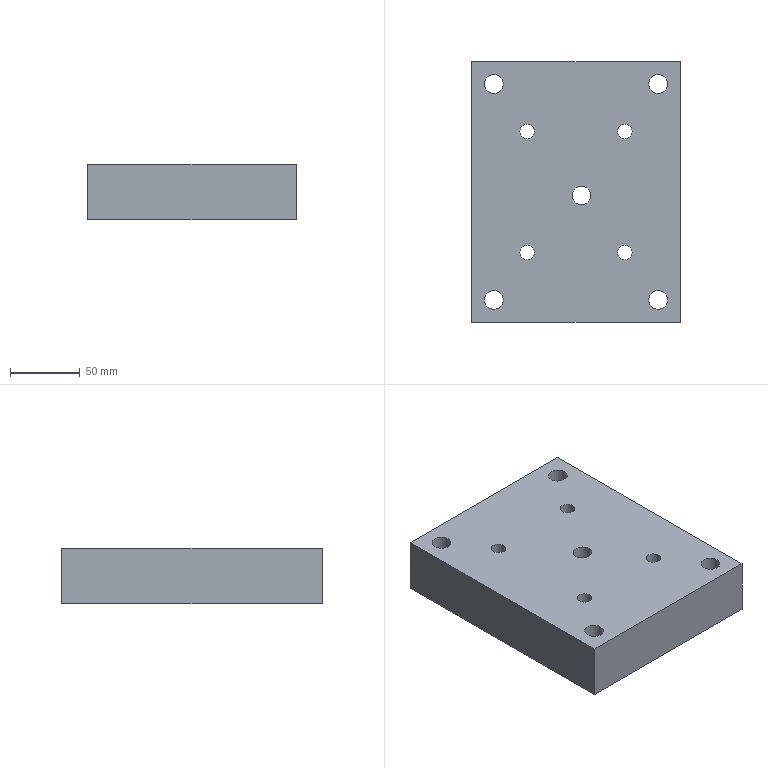Part | STEP file | lll_id2198_x_t | 1 solid | 47 faces | box 150 x 187 x 40 mm | volume 927967 mm3 | cylinder 24 | plane 21 | cone 2 | commonest cylinder face diameters 10 x8 13.509 x5 20.007 x5 10.506 x4 10.505 x2
STEP:
#1=CARTESIAN_POINT('',(2920.,63.439,117.5));
#2=VERTEX_POINT('',#1);
#3=CARTESIAN_POINT('',(2928.371,68.5,117.5));
#4=VERTEX_POINT('',#3);
#5=CARTESIAN_POINT('',(2923.648,66.859,117.5));
#6=DIRECTION('',(0.,0.,-1.));
#7=DIRECTION('',(-1.,0.,0.));
#8=AXIS2_PLACEMENT_3D('',#5,#6,#7);
#9=CIRCLE('',#8,5.);
#10=EDGE_CURVE('',#2,#4,#9,.T.);
#11=ORIENTED_EDGE('',*,*,#10,.F.);
#12=CARTESIAN_POINT('',(2920.,28.561,117.5));
#13=VERTEX_POINT('',#12);
#14=CARTESIAN_POINT('',(2920.,0.00007422,117.5));
#15=DIRECTION('',(0.,1.,0.));
#16=VECTOR('',#15,1.);
#17=LINE('',#14,#16);
#18=EDGE_CURVE('',#13,#2,#17,.T.);
#19=ORIENTED_EDGE('',*,*,#18,.F.);
#20=CARTESIAN_POINT('',(2928.371,23.5,117.5));
#21=VERTEX_POINT('',#20);
#22=CARTESIAN_POINT('',(2923.648,25.142,117.5));
#23=DIRECTION('',(0.,0.,-1.));
#24=DIRECTION('',(-1.,0.,0.));
#25=AXIS2_PLACEMENT_3D('',#22,#23,#24);
#26=CIRCLE('',#25,5.);
#27=EDGE_CURVE('',#21,#13,#26,.T.);
#28=ORIENTED_EDGE('',*,*,#27,.F.);
#29=CARTESIAN_POINT('',(3011.629,23.5,117.5));
#30=VERTEX_POINT('',#29);
#31=CARTESIAN_POINT('',(2970.,23.5,117.5));
#32=DIRECTION('',(-1.,0.,0.));
#33=VECTOR('',#32,1.);
#34=LINE('',#31,#33);
#35=EDGE_CURVE('',#30,#21,#34,.T.);
#36=ORIENTED_EDGE('',*,*,#35,.F.);
#37=CARTESIAN_POINT('',(3020.,28.561,117.5));
#38=VERTEX_POINT('',#37);
#39=CARTESIAN_POINT('',(3016.352,25.142,117.5));
#40=DIRECTION('',(0.,0.,-1.));
#41=DIRECTION('',(-1.,0.,0.));
#42=AXIS2_PLACEMENT_3D('',#39,#40,#41);
#43=CIRCLE('',#42,5.);
#44=EDGE_CURVE('',#38,#30,#43,.T.);
#45=ORIENTED_EDGE('',*,*,#44,.F.);
#46=CARTESIAN_POINT('',(3020.,63.439,117.5));
#47=VERTEX_POINT('',#46);
#48=CARTESIAN_POINT('',(3020.,0.00007422,117.5));
#49=DIRECTION('',(0.,-1.,0.));
#50=VECTOR('',#49,1.);
#51=LINE('',#48,#50);
#52=EDGE_CURVE('',#47,#38,#51,.T.);
#53=ORIENTED_EDGE('',*,*,#52,.F.);
#54=CARTESIAN_POINT('',(3011.629,68.5,117.5));
#55=VERTEX_POINT('',#54);
#56=CARTESIAN_POINT('',(3016.352,66.859,117.5));
#57=DIRECTION('',(0.,0.,-1.));
#58=DIRECTION('',(-1.,0.,0.));
#59=AXIS2_PLACEMENT_3D('',#56,#57,#58);
#60=CIRCLE('',#59,5.);
#61=EDGE_CURVE('',#55,#47,#60,.T.);
#62=ORIENTED_EDGE('',*,*,#61,.F.);
#63=CARTESIAN_POINT('',(2970.,68.5,117.5));
#64=DIRECTION('',(1.,0.,0.));
#65=VECTOR('',#64,1.);
#66=LINE('',#63,#65);
#67=EDGE_CURVE('',#4,#55,#66,.T.);
#68=ORIENTED_EDGE('',*,*,#67,.F.);
#69=EDGE_LOOP('',(#11,#19,#28,#36,#45,#53,#62,#68));
#70=FACE_BOUND('',#69,.T.);
#71=CARTESIAN_POINT('',(2920.,-28.561,117.5));
#72=VERTEX_POINT('',#71);
#73=CARTESIAN_POINT('',(2928.371,-23.5,117.5));
#74=VERTEX_POINT('',#73);
#75=CARTESIAN_POINT('',(2923.648,-25.141,117.5));
#76=DIRECTION('',(0.,0.,-1.));
#77=DIRECTION('',(-1.,0.,0.));
#78=AXIS2_PLACEMENT_3D('',#75,#76,#77);
#79=CIRCLE('',#78,5.);
#80=EDGE_CURVE('',#72,#74,#79,.T.);
#81=ORIENTED_EDGE('',*,*,#80,.F.);
#82=CARTESIAN_POINT('',(2920.,-63.439,117.5));
#83=VERTEX_POINT('',#82);
#84=CARTESIAN_POINT('',(2920.,0.00007422,117.5));
#85=DIRECTION('',(0.,1.,0.));
#86=VECTOR('',#85,1.);
#87=LINE('',#84,#86);
#88=EDGE_CURVE('',#83,#72,#87,.T.);
#89=ORIENTED_EDGE('',*,*,#88,.F.);
#90=CARTESIAN_POINT('',(2928.371,-68.5,117.5));
#91=VERTEX_POINT('',#90);
#92=CARTESIAN_POINT('',(2923.648,-66.858,117.5));
#93=DIRECTION('',(0.,0.,-1.));
#94=DIRECTION('',(-1.,0.,0.));
#95=AXIS2_PLACEMENT_3D('',#92,#93,#94);
#96=CIRCLE('',#95,5.);
#97=EDGE_CURVE('',#91,#83,#96,.T.);
#98=ORIENTED_EDGE('',*,*,#97,.F.);
#99=CARTESIAN_POINT('',(3011.629,-68.5,117.5));
#100=VERTEX_POINT('',#99);
#101=CARTESIAN_POINT('',(2970.,-68.5,117.5));
#102=DIRECTION('',(-1.,0.,0.));
#103=VECTOR('',#102,1.);
#104=LINE('',#101,#103);
#105=EDGE_CURVE('',#100,#91,#104,.T.);
#106=ORIENTED_EDGE('',*,*,#105,.F.);
#107=CARTESIAN_POINT('',(3020.,-63.439,117.5));
#108=VERTEX_POINT('',#107);
#109=CARTESIAN_POINT('',(3016.352,-66.858,117.5));
#110=DIRECTION('',(0.,0.,-1.));
#111=DIRECTION('',(-1.,0.,0.));
#112=AXIS2_PLACEMENT_3D('',#109,#110,#111);
#113=CIRCLE('',#112,5.);
#114=EDGE_CURVE('',#108,#100,#113,.T.);
#115=ORIENTED_EDGE('',*,*,#114,.F.);
#116=CARTESIAN_POINT('',(3020.,-28.561,117.5));
#117=VERTEX_POINT('',#116);
#118=CARTESIAN_POINT('',(3020.,0.00007422,117.5));
#119=DIRECTION('',(0.,-1.,0.));
#120=VECTOR('',#119,1.);
#121=LINE('',#118,#120);
#122=EDGE_CURVE('',#117,#108,#121,.T.);
#123=ORIENTED_EDGE('',*,*,#122,.F.);
#124=CARTESIAN_POINT('',(3011.629,-23.5,117.5));
#125=VERTEX_POINT('',#124);
#126=CARTESIAN_POINT('',(3016.352,-25.141,117.5));
#127=DIRECTION('',(0.,0.,-1.));
#128=DIRECTION('',(-1.,0.,0.));
#129=AXIS2_PLACEMENT_3D('',#126,#127,#128);
#130=CIRCLE('',#129,5.);
#131=EDGE_CURVE('',#125,#117,#130,.T.);
#132=ORIENTED_EDGE('',*,*,#131,.F.);
#133=CARTESIAN_POINT('',(2970.,-23.5,117.5));
#134=DIRECTION('',(1.,0.,0.));
#135=VECTOR('',#134,1.);
#136=LINE('',#133,#135);
#137=EDGE_CURVE('',#74,#125,#136,.T.);
#138=ORIENTED_EDGE('',*,*,#137,.F.);
#139=EDGE_LOOP('',(#81,#89,#98,#106,#115,#123,#132,#138));
#140=FACE_BOUND('',#139,.T.);
#141=CARTESIAN_POINT('',(2935.747,77.5,117.5));
#142=VERTEX_POINT('',#141);
#143=CARTESIAN_POINT('',(2941.,77.5,117.5));
#144=DIRECTION('',(0.,0.,-1.));
#145=DIRECTION('',(-1.,0.,0.));
#146=AXIS2_PLACEMENT_3D('',#143,#144,#145);
#147=CIRCLE('',#146,5.253);
#148=EDGE_CURVE('',#142,#142,#147,.T.);
#149=ORIENTED_EDGE('',*,*,#148,.F.);
#150=EDGE_LOOP('',(#149));
#151=FACE_BOUND('',#150,.T.);
#152=CARTESIAN_POINT('',(3039.003,77.5,117.5));
#153=VERTEX_POINT('',#152);
#154=CARTESIAN_POINT('',(3029.,77.5,117.5));
#155=DIRECTION('',(0.,0.,1.));
#156=DIRECTION('',(1.,0.,0.));
#157=AXIS2_PLACEMENT_3D('',#154,#155,#156);
#158=CIRCLE('',#157,10.004);
#159=EDGE_CURVE('',#153,#153,#158,.T.);
#160=ORIENTED_EDGE('',*,*,#159,.T.);
#161=EDGE_LOOP('',(#160));
#162=FACE_BOUND('',#161,.T.);
#163=CARTESIAN_POINT('',(2921.003,-77.5,117.5));
#164=VERTEX_POINT('',#163);
#165=CARTESIAN_POINT('',(2911.,-77.5,117.5));
#166=DIRECTION('',(0.,0.,1.));
#167=DIRECTION('',(1.,0.,0.));
#168=AXIS2_PLACEMENT_3D('',#165,#166,#167);
#169=CIRCLE('',#168,10.004);
#170=EDGE_CURVE('',#164,#164,#169,.T.);
#171=ORIENTED_EDGE('',*,*,#170,.T.);
#172=EDGE_LOOP('',(#171));
#173=FACE_BOUND('',#172,.T.);
#174=CARTESIAN_POINT('',(2993.747,-77.5,117.5));
#175=VERTEX_POINT('',#174);
#176=CARTESIAN_POINT('',(2999.,-77.5,117.5));
#177=DIRECTION('',(0.,0.,-1.));
#178=DIRECTION('',(-1.,0.,0.));
#179=AXIS2_PLACEMENT_3D('',#176,#177,#178);
#180=CIRCLE('',#179,5.253);
#181=EDGE_CURVE('',#175,#175,#180,.T.);
#182=ORIENTED_EDGE('',*,*,#181,.F.);
#183=EDGE_LOOP('',(#182));
#184=FACE_BOUND('',#183,.T.);
#185=CARTESIAN_POINT('',(3045.,-93.5,117.5));
#186=VERTEX_POINT('',#185);
#187=CARTESIAN_POINT('',(3045.,93.5,117.5));
#188=VERTEX_POINT('',#187);
#189=CARTESIAN_POINT('',(3045.,0.00007422,117.5));
#190=DIRECTION('',(0.,1.,0.));
#191=VECTOR('',#190,1.);
#192=LINE('',#189,#191);
#193=EDGE_CURVE('',#186,#188,#192,.T.);
#194=ORIENTED_EDGE('',*,*,#193,.F.);
#195=CARTESIAN_POINT('',(2895.,-93.5,117.5));
#196=VERTEX_POINT('',#195);
#197=CARTESIAN_POINT('',(2970.,-93.5,117.5));
#198=DIRECTION('',(1.,0.,0.));
#199=VECTOR('',#198,1.);
#200=LINE('',#197,#199);
#201=EDGE_CURVE('',#196,#186,#200,.T.);
#202=ORIENTED_EDGE('',*,*,#201,.F.);
#203=CARTESIAN_POINT('',(2895.,93.5,117.5));
#204=VERTEX_POINT('',#203);
#205=CARTESIAN_POINT('',(2895.,0.00007422,117.5));
#206=DIRECTION('',(0.,-1.,0.));
#207=VECTOR('',#206,1.);
#208=LINE('',#205,#207);
#209=EDGE_CURVE('',#204,#196,#208,.T.);
#210=ORIENTED_EDGE('',*,*,#209,.F.);
#211=CARTESIAN_POINT('',(2970.,93.5,117.5));
#212=DIRECTION('',(-1.,0.,0.));
#213=VECTOR('',#212,1.);
#214=LINE('',#211,#213);
#215=EDGE_CURVE('',#188,#204,#214,.T.);
#216=ORIENTED_EDGE('',*,*,#215,.F.);
#217=EDGE_LOOP('',(#194,#202,#210,#216));
#218=FACE_BOUND('',#217,.T.);
#219=CARTESIAN_POINT('',(3039.003,-77.5,117.5));
#220=VERTEX_POINT('',#219);
#221=CARTESIAN_POINT('',(3029.,-77.5,117.5));
#222=DIRECTION('',(0.,0.,1.));
#223=DIRECTION('',(1.,0.,0.));
#224=AXIS2_PLACEMENT_3D('',#221,#222,#223);
#225=CIRCLE('',#224,10.004);
#226=EDGE_CURVE('',#220,#220,#225,.T.);
#227=ORIENTED_EDGE('',*,*,#226,.T.);
#228=EDGE_LOOP('',(#227));
#229=FACE_BOUND('',#228,.T.);
#230=CARTESIAN_POINT('',(2984.003,-2.5,117.5));
#231=VERTEX_POINT('',#230);
#232=CARTESIAN_POINT('',(2974.,-2.5,117.5));
#233=DIRECTION('',(0.,0.,1.));
#234=DIRECTION('',(1.,0.,0.));
#235=AXIS2_PLACEMENT_3D('',#232,#233,#234);
#236=CIRCLE('',#235,10.004);
#237=EDGE_CURVE('',#231,#231,#236,.T.);
#238=ORIENTED_EDGE('',*,*,#237,.T.);
#239=EDGE_LOOP('',(#238));
#240=FACE_BOUND('',#239,.T.);
#241=CARTESIAN_POINT('',(2921.003,77.5,117.5));
#242=VERTEX_POINT('',#241);
#243=CARTESIAN_POINT('',(2911.,77.5,117.5));
#244=DIRECTION('',(0.,0.,1.));
#245=DIRECTION('',(1.,0.,0.));
#246=AXIS2_PLACEMENT_3D('',#243,#244,#245);
#247=CIRCLE('',#246,10.004);
#248=EDGE_CURVE('',#242,#242,#247,.T.);
#249=ORIENTED_EDGE('',*,*,#248,.T.);
#250=EDGE_LOOP('',(#249));
#251=FACE_BOUND('',#250,.T.);
#252=CARTESIAN_POINT('',(2970.,0.00007422,117.5));
#253=DIRECTION('',(0.,0.,-1.));
#254=DIRECTION('',(-1.,0.,0.));
#255=AXIS2_PLACEMENT_3D('',#252,#253,#254);
#256=PLANE('',#255);
#257=ADVANCED_FACE('',(#70,#140,#151,#162,#173,#184,#218,#229,#240,#251),#256,.T.);
#258=CARTESIAN_POINT('',(2999.747,43.5,157.5));
#259=VERTEX_POINT('',#258);
#260=CARTESIAN_POINT('',(3005.,43.5,157.5));
#261=DIRECTION('',(0.,0.,-1.));
#262=DIRECTION('',(-1.,0.,0.));
#263=AXIS2_PLACEMENT_3D('',#260,#261,#262);
#264=CIRCLE('',#263,5.253);
#265=EDGE_CURVE('',#259,#259,#264,.T.);
#266=ORIENTED_EDGE('',*,*,#265,.T.);
#267=EDGE_LOOP('',(#266));
#268=FACE_BOUND('',#267,.T.);
#269=CARTESIAN_POINT('',(2929.747,43.5,157.5));
#270=VERTEX_POINT('',#269);
#271=CARTESIAN_POINT('',(2935.,43.5,157.5));
#272=DIRECTION('',(0.,0.,-1.));
#273=DIRECTION('',(-1.,0.,0.));
#274=AXIS2_PLACEMENT_3D('',#271,#272,#273);
#275=CIRCLE('',#274,5.253);
#276=EDGE_CURVE('',#270,#270,#275,.T.);
#277=ORIENTED_EDGE('',*,*,#276,.T.);
#278=EDGE_LOOP('',(#277));
#279=FACE_BOUND('',#278,.T.);
#280=CARTESIAN_POINT('',(2999.747,-43.5,157.5));
#281=VERTEX_POINT('',#280);
#282=CARTESIAN_POINT('',(3005.,-43.5,157.5));
#283=DIRECTION('',(0.,0.,-1.));
#284=DIRECTION('',(-1.,0.,0.));
#285=AXIS2_PLACEMENT_3D('',#282,#283,#284);
#286=CIRCLE('',#285,5.253);
#287=EDGE_CURVE('',#281,#281,#286,.T.);
#288=ORIENTED_EDGE('',*,*,#287,.T.);
#289=EDGE_LOOP('',(#288));
#290=FACE_BOUND('',#289,.T.);
#291=CARTESIAN_POINT('',(2929.747,-43.5,157.5));
#292=VERTEX_POINT('',#291);
#293=CARTESIAN_POINT('',(2935.,-43.5,157.5));
#294=DIRECTION('',(0.,0.,-1.));
#295=DIRECTION('',(-1.,0.,0.));
#296=AXIS2_PLACEMENT_3D('',#293,#294,#295);
#297=CIRCLE('',#296,5.253);
#298=EDGE_CURVE('',#292,#292,#297,.T.);
#299=ORIENTED_EDGE('',*,*,#298,.T.);
#300=EDGE_LOOP('',(#299));
#301=FACE_BOUND('',#300,.T.);
#302=CARTESIAN_POINT('',(2904.245,77.5,157.5));
#303=VERTEX_POINT('',#302);
#304=CARTESIAN_POINT('',(2911.,77.5,157.5));
#305=DIRECTION('',(0.,0.,1.));
#306=DIRECTION('',(-1.,0.,0.));
#307=AXIS2_PLACEMENT_3D('',#304,#305,#306);
#308=CIRCLE('',#307,6.755);
#309=EDGE_CURVE('',#303,#303,#308,.T.);
#310=ORIENTED_EDGE('',*,*,#309,.F.);
#311=EDGE_LOOP('',(#310));
#312=FACE_BOUND('',#311,.T.);
#313=CARTESIAN_POINT('',(3022.245,77.5,157.5));
#314=VERTEX_POINT('',#313);
#315=CARTESIAN_POINT('',(3029.,77.5,157.5));
#316=DIRECTION('',(0.,0.,1.));
#317=DIRECTION('',(-1.,0.,0.));
#318=AXIS2_PLACEMENT_3D('',#315,#316,#317);
#319=CIRCLE('',#318,6.755);
#320=EDGE_CURVE('',#314,#314,#319,.T.);
#321=ORIENTED_EDGE('',*,*,#320,.F.);
#322=EDGE_LOOP('',(#321));
#323=FACE_BOUND('',#322,.T.);
#324=CARTESIAN_POINT('',(2967.245,-2.5,157.5));
#325=VERTEX_POINT('',#324);
#326=CARTESIAN_POINT('',(2974.,-2.5,157.5));
#327=DIRECTION('',(0.,0.,1.));
#328=DIRECTION('',(-1.,0.,0.));
#329=AXIS2_PLACEMENT_3D('',#326,#327,#328);
#330=CIRCLE('',#329,6.755);
#331=EDGE_CURVE('',#325,#325,#330,.T.);
#332=ORIENTED_EDGE('',*,*,#331,.F.);
#333=EDGE_LOOP('',(#332));
#334=FACE_BOUND('',#333,.T.);
#335=CARTESIAN_POINT('',(2904.245,-77.5,157.5));
#336=VERTEX_POINT('',#335);
#337=CARTESIAN_POINT('',(2911.,-77.5,157.5));
#338=DIRECTION('',(0.,0.,1.));
#339=DIRECTION('',(-1.,0.,0.));
#340=AXIS2_PLACEMENT_3D('',#337,#338,#339);
#341=CIRCLE('',#340,6.755);
#342=EDGE_CURVE('',#336,#336,#341,.T.);
#343=ORIENTED_EDGE('',*,*,#342,.F.);
#344=EDGE_LOOP('',(#343));
#345=FACE_BOUND('',#344,.T.);
#346=CARTESIAN_POINT('',(3022.245,-77.5,157.5));
#347=VERTEX_POINT('',#346);
#348=CARTESIAN_POINT('',(3029.,-77.5,157.5));
#349=DIRECTION('',(0.,0.,1.));
#350=DIRECTION('',(-1.,0.,0.));
#351=AXIS2_PLACEMENT_3D('',#348,#349,#350);
#352=CIRCLE('',#351,6.755);
#353=EDGE_CURVE('',#347,#347,#352,.T.);
#354=ORIENTED_EDGE('',*,*,#353,.F.);
#355=EDGE_LOOP('',(#354));
#356=FACE_BOUND('',#355,.T.);
#357=CARTESIAN_POINT('',(3045.,-93.5,157.5));
#358=VERTEX_POINT('',#357);
#359=CARTESIAN_POINT('',(2895.,-93.5,157.5));
#360=VERTEX_POINT('',#359);
#361=CARTESIAN_POINT('',(2970.,-93.5,157.5));
#362=DIRECTION('',(-1.,0.,0.));
#363=VECTOR('',#362,1.);
#364=LINE('',#361,#363);
#365=EDGE_CURVE('',#358,#360,#364,.T.);
#366=ORIENTED_EDGE('',*,*,#365,.F.);
#367=CARTESIAN_POINT('',(3045.,93.5,157.5));
#368=VERTEX_POINT('',#367);
#369=CARTESIAN_POINT('',(3045.,0.00007422,157.5));
#370=DIRECTION('',(0.,-1.,0.));
#371=VECTOR('',#370,1.);
#372=LINE('',#369,#371);
#373=EDGE_CURVE('',#368,#358,#372,.T.);
#374=ORIENTED_EDGE('',*,*,#373,.F.);
#375=CARTESIAN_POINT('',(2895.,93.5,157.5));
#376=VERTEX_POINT('',#375);
#377=CARTESIAN_POINT('',(2970.,93.5,157.5));
#378=DIRECTION('',(1.,0.,0.));
#379=VECTOR('',#378,1.);
#380=LINE('',#377,#379);
#381=EDGE_CURVE('',#376,#368,#380,.T.);
#382=ORIENTED_EDGE('',*,*,#381,.F.);
#383=CARTESIAN_POINT('',(2895.,0.00007422,157.5));
#384=DIRECTION('',(0.,1.,0.));
#385=VECTOR('',#384,1.);
#386=LINE('',#383,#385);
#387=EDGE_CURVE('',#360,#376,#386,.T.);
#388=ORIENTED_EDGE('',*,*,#387,.F.);
#389=EDGE_LOOP('',(#366,#374,#382,#388));
#390=FACE_BOUND('',#389,.T.);
#391=CARTESIAN_POINT('',(-2196.249,0.,157.5));
#392=DIRECTION('',(0.,0.,-1.));
#393=DIRECTION('',(1.,0.,0.));
#394=AXIS2_PLACEMENT_3D('',#391,#392,#393);
#395=PLANE('',#394);
#396=ADVANCED_FACE('',(#268,#279,#290,#301,#312,#323,#334,#345,#356,#390),#395,.F.);
#397=CARTESIAN_POINT('',(3045.,-93.5,127.5));
#398=DIRECTION('',(0.,0.,1.));
#399=VECTOR('',#398,1.);
#400=LINE('',#397,#399);
#401=EDGE_CURVE('',#186,#358,#400,.T.);
#402=ORIENTED_EDGE('',*,*,#401,.T.);
#403=ORIENTED_EDGE('',*,*,#365,.T.);
#404=CARTESIAN_POINT('',(2895.,-93.5,127.5));
#405=DIRECTION('',(0.,0.,1.));
#406=VECTOR('',#405,1.);
#407=LINE('',#404,#406);
#408=EDGE_CURVE('',#196,#360,#407,.T.);
#409=ORIENTED_EDGE('',*,*,#408,.F.);
#410=ORIENTED_EDGE('',*,*,#201,.T.);
#411=EDGE_LOOP('',(#402,#403,#409,#410));
#412=FACE_OUTER_BOUND('',#411,.T.);
#413=CARTESIAN_POINT('',(2970.,-93.5,127.5));
#414=DIRECTION('',(0.,-1.,0.));
#415=DIRECTION('',(0.,0.,-1.));
#416=AXIS2_PLACEMENT_3D('',#413,#414,#415);
#417=PLANE('',#416);
#418=ADVANCED_FACE('',(#412),#417,.T.);
#419=ORIENTED_EDGE('',*,*,#408,.T.);
#420=ORIENTED_EDGE('',*,*,#387,.T.);
#421=CARTESIAN_POINT('',(2895.,93.5,127.5));
#422=DIRECTION('',(0.,0.,1.));
#423=VECTOR('',#422,1.);
#424=LINE('',#421,#423);
#425=EDGE_CURVE('',#204,#376,#424,.T.);
#426=ORIENTED_EDGE('',*,*,#425,.F.);
#427=ORIENTED_EDGE('',*,*,#209,.T.);
#428=EDGE_LOOP('',(#419,#420,#426,#427));
#429=FACE_OUTER_BOUND('',#428,.T.);
#430=CARTESIAN_POINT('',(2895.,0.00007422,127.5));
#431=DIRECTION('',(-1.,0.,0.));
#432=DIRECTION('',(0.,0.,1.));
#433=AXIS2_PLACEMENT_3D('',#430,#431,#432);
#434=PLANE('',#433);
#435=ADVANCED_FACE('',(#429),#434,.T.);
#436=ORIENTED_EDGE('',*,*,#425,.T.);
#437=ORIENTED_EDGE('',*,*,#381,.T.);
#438=CARTESIAN_POINT('',(3045.,93.5,127.5));
#439=DIRECTION('',(0.,0.,1.));
#440=VECTOR('',#439,1.);
#441=LINE('',#438,#440);
#442=EDGE_CURVE('',#188,#368,#441,.T.);
#443=ORIENTED_EDGE('',*,*,#442,.F.);
#444=ORIENTED_EDGE('',*,*,#215,.T.);
#445=EDGE_LOOP('',(#436,#437,#443,#444));
#446=FACE_OUTER_BOUND('',#445,.T.);
#447=CARTESIAN_POINT('',(2970.,93.5,127.5));
#448=DIRECTION('',(0.,1.,0.));
#449=DIRECTION('',(0.,0.,1.));
#450=AXIS2_PLACEMENT_3D('',#447,#448,#449);
#451=PLANE('',#450);
#452=ADVANCED_FACE('',(#446),#451,.T.);
#453=ORIENTED_EDGE('',*,*,#193,.T.);
#454=ORIENTED_EDGE('',*,*,#442,.T.);
#455=ORIENTED_EDGE('',*,*,#373,.T.);
#456=ORIENTED_EDGE('',*,*,#401,.F.);
#457=EDGE_LOOP('',(#453,#454,#455,#456));
#458=FACE_OUTER_BOUND('',#457,.T.);
#459=CARTESIAN_POINT('',(3045.,0.00007422,127.5));
#460=DIRECTION('',(1.,0.,0.));
#461=DIRECTION('',(0.,0.,-1.));
#462=AXIS2_PLACEMENT_3D('',#459,#460,#461);
#463=PLANE('',#462);
#464=ADVANCED_FACE('',(#458),#463,.T.);
#465=ORIENTED_EDGE('',*,*,#353,.T.);
#466=EDGE_LOOP('',(#465));
#467=FACE_BOUND('',#466,.T.);
#468=CARTESIAN_POINT('',(3035.755,-77.5,132.5));
#469=VERTEX_POINT('',#468);
#470=CARTESIAN_POINT('',(3029.,-77.5,132.5));
#471=DIRECTION('',(0.,0.,1.));
#472=DIRECTION('',(1.,0.,0.));
#473=AXIS2_PLACEMENT_3D('',#470,#471,#472);
#474=CIRCLE('',#473,6.755);
#475=EDGE_CURVE('',#469,#469,#474,.T.);
#476=ORIENTED_EDGE('',*,*,#475,.F.);
#477=EDGE_LOOP('',(#476));
#478=FACE_BOUND('',#477,.T.);
#479=CARTESIAN_POINT('',(3029.,-77.5,112.5));
#480=DIRECTION('',(0.,0.,1.));
#481=DIRECTION('',(1.,0.,0.));
#482=AXIS2_PLACEMENT_3D('',#479,#480,#481);
#483=CYLINDRICAL_SURFACE('',#482,6.755);
#484=ADVANCED_FACE('',(#467,#478),#483,.F.);
#485=ORIENTED_EDGE('',*,*,#475,.T.);
#486=EDGE_LOOP('',(#485));
#487=FACE_BOUND('',#486,.T.);
#488=CARTESIAN_POINT('',(3039.003,-77.5,132.5));
#489=VERTEX_POINT('',#488);
#490=CARTESIAN_POINT('',(3029.,-77.5,132.5));
#491=DIRECTION('',(0.,0.,1.));
#492=DIRECTION('',(1.,0.,0.));
#493=AXIS2_PLACEMENT_3D('',#490,#491,#492);
#494=CIRCLE('',#493,10.004);
#495=EDGE_CURVE('',#489,#489,#494,.T.);
#496=ORIENTED_EDGE('',*,*,#495,.F.);
#497=EDGE_LOOP('',(#496));
#498=FACE_BOUND('',#497,.T.);
#499=CARTESIAN_POINT('',(3029.,-77.5,132.5));
#500=DIRECTION('',(0.,0.,1.));
#501=DIRECTION('',(1.,0.,0.));
#502=AXIS2_PLACEMENT_3D('',#499,#500,#501);
#503=PLANE('',#502);
#504=ADVANCED_FACE('',(#487,#498),#503,.F.);
#505=ORIENTED_EDGE('',*,*,#495,.T.);
#506=EDGE_LOOP('',(#505));
#507=FACE_BOUND('',#506,.T.);
#508=ORIENTED_EDGE('',*,*,#226,.F.);
#509=EDGE_LOOP('',(#508));
#510=FACE_BOUND('',#509,.T.);
#511=CARTESIAN_POINT('',(3029.,-77.5,117.5));
#512=DIRECTION('',(0.,0.,1.));
#513=DIRECTION('',(1.,0.,0.));
#514=AXIS2_PLACEMENT_3D('',#511,#512,#513);
#515=CYLINDRICAL_SURFACE('',#514,10.004);
#516=ADVANCED_FACE('',(#507,#510),#515,.F.);
#517=ORIENTED_EDGE('',*,*,#181,.T.);
#518=EDGE_LOOP('',(#517));
#519=FACE_BOUND('',#518,.T.);
#520=CARTESIAN_POINT('',(3004.253,-77.5,147.254));
#521=VERTEX_POINT('',#520);
#522=CARTESIAN_POINT('',(2999.,-77.5,147.254));
#523=DIRECTION('',(0.,0.,1.));
#524=DIRECTION('',(1.,0.,0.));
#525=AXIS2_PLACEMENT_3D('',#522,#523,#524);
#526=CIRCLE('',#525,5.253);
#527=EDGE_CURVE('',#521,#521,#526,.T.);
#528=ORIENTED_EDGE('',*,*,#527,.T.);
#529=EDGE_LOOP('',(#528));
#530=FACE_BOUND('',#529,.T.);
#531=CARTESIAN_POINT('',(2999.,-77.5,112.5));
#532=DIRECTION('',(0.,0.,1.));
#533=DIRECTION('',(1.,0.,0.));
#534=AXIS2_PLACEMENT_3D('',#531,#532,#533);
#535=CYLINDRICAL_SURFACE('',#534,5.253);
#536=ADVANCED_FACE('',(#519,#530),#535,.F.);
#537=CARTESIAN_POINT('',(2999.,-77.5,152.506));
#538=VERTEX_POINT('',#537);
#539=VERTEX_LOOP('',#538);
#540=FACE_BOUND('',#539,.T.);
#541=ORIENTED_EDGE('',*,*,#527,.F.);
#542=EDGE_LOOP('',(#541));
#543=FACE_BOUND('',#542,.T.);
#544=CARTESIAN_POINT('',(2999.,-77.5,147.254));
#545=DIRECTION('',(0.,0.,-1.));
#546=DIRECTION('',(-1.,0.,0.));
#547=AXIS2_PLACEMENT_3D('',#544,#545,#546);
#548=CONICAL_SURFACE('',#547,5.253,45.);
#549=ADVANCED_FACE('',(#540,#543),#548,.F.);
#550=ORIENTED_EDGE('',*,*,#342,.T.);
#551=EDGE_LOOP('',(#550));
#552=FACE_BOUND('',#551,.T.);
#553=CARTESIAN_POINT('',(2917.755,-77.5,132.5));
#554=VERTEX_POINT('',#553);
#555=CARTESIAN_POINT('',(2911.,-77.5,132.5));
#556=DIRECTION('',(0.,0.,1.));
#557=DIRECTION('',(1.,0.,0.));
#558=AXIS2_PLACEMENT_3D('',#555,#556,#557);
#559=CIRCLE('',#558,6.755);
#560=EDGE_CURVE('',#554,#554,#559,.T.);
#561=ORIENTED_EDGE('',*,*,#560,.F.);
#562=EDGE_LOOP('',(#561));
#563=FACE_BOUND('',#562,.T.);
#564=CARTESIAN_POINT('',(2911.,-77.5,112.5));
#565=DIRECTION('',(0.,0.,1.));
#566=DIRECTION('',(1.,0.,0.));
#567=AXIS2_PLACEMENT_3D('',#564,#565,#566);
#568=CYLINDRICAL_SURFACE('',#567,6.755);
#569=ADVANCED_FACE('',(#552,#563),#568,.F.);
#570=ORIENTED_EDGE('',*,*,#560,.T.);
#571=EDGE_LOOP('',(#570));
#572=FACE_BOUND('',#571,.T.);
#573=CARTESIAN_POINT('',(2921.003,-77.5,132.5));
#574=VERTEX_POINT('',#573);
#575=CARTESIAN_POINT('',(2911.,-77.5,132.5));
#576=DIRECTION('',(0.,0.,1.));
#577=DIRECTION('',(1.,0.,0.));
#578=AXIS2_PLACEMENT_3D('',#575,#576,#577);
#579=CIRCLE('',#578,10.004);
#580=EDGE_CURVE('',#574,#574,#579,.T.);
#581=ORIENTED_EDGE('',*,*,#580,.F.);
#582=EDGE_LOOP('',(#581));
#583=FACE_BOUND('',#582,.T.);
#584=CARTESIAN_POINT('',(2911.,-77.5,132.5));
#585=DIRECTION('',(0.,0.,1.));
#586=DIRECTION('',(1.,0.,0.));
#587=AXIS2_PLACEMENT_3D('',#584,#585,#586);
#588=PLANE('',#587);
#589=ADVANCED_FACE('',(#572,#583),#588,.F.);
#590=ORIENTED_EDGE('',*,*,#580,.T.);
#591=EDGE_LOOP('',(#590));
#592=FACE_BOUND('',#591,.T.);
#593=ORIENTED_EDGE('',*,*,#170,.F.);
#594=EDGE_LOOP('',(#593));
#595=FACE_BOUND('',#594,.T.);
#596=CARTESIAN_POINT('',(2911.,-77.5,117.5));
#597=DIRECTION('',(0.,0.,1.));
#598=DIRECTION('',(1.,0.,0.));
#599=AXIS2_PLACEMENT_3D('',#596,#597,#598);
#600=CYLINDRICAL_SURFACE('',#599,10.004);
#601=ADVANCED_FACE('',(#592,#595),#600,.F.);
#602=ORIENTED_EDGE('',*,*,#331,.T.);
#603=EDGE_LOOP('',(#602));
#604=FACE_BOUND('',#603,.T.);
#605=CARTESIAN_POINT('',(2980.755,-2.5,132.5));
#606=VERTEX_POINT('',#605);
#607=CARTESIAN_POINT('',(2974.,-2.5,132.5));
#608=DIRECTION('',(0.,0.,1.));
#609=DIRECTION('',(1.,0.,0.));
#610=AXIS2_PLACEMENT_3D('',#607,#608,#609);
#611=CIRCLE('',#610,6.755);
#612=EDGE_CURVE('',#606,#606,#611,.T.);
#613=ORIENTED_EDGE('',*,*,#612,.F.);
#614=EDGE_LOOP('',(#613));
#615=FACE_BOUND('',#614,.T.);
#616=CARTESIAN_POINT('',(2974.,-2.5,112.5));
#617=DIRECTION('',(0.,0.,1.));
#618=DIRECTION('',(1.,0.,0.));
#619=AXIS2_PLACEMENT_3D('',#616,#617,#618);
#620=CYLINDRICAL_SURFACE('',#619,6.755);
#621=ADVANCED_FACE('',(#604,#615),#620,.F.);
#622=ORIENTED_EDGE('',*,*,#612,.T.);
#623=EDGE_LOOP('',(#622));
#624=FACE_BOUND('',#623,.T.);
#625=CARTESIAN_POINT('',(2984.003,-2.5,132.5));
#626=VERTEX_POINT('',#625);
#627=CARTESIAN_POINT('',(2974.,-2.5,132.5));
#628=DIRECTION('',(0.,0.,1.));
#629=DIRECTION('',(1.,0.,0.));
#630=AXIS2_PLACEMENT_3D('',#627,#628,#629);
#631=CIRCLE('',#630,10.004);
#632=EDGE_CURVE('',#626,#626,#631,.T.);
#633=ORIENTED_EDGE('',*,*,#632,.F.);
#634=EDGE_LOOP('',(#633));
#635=FACE_BOUND('',#634,.T.);
#636=CARTESIAN_POINT('',(2974.,-2.5,132.5));
#637=DIRECTION('',(0.,0.,1.));
#638=DIRECTION('',(1.,0.,0.));
#639=AXIS2_PLACEMENT_3D('',#636,#637,#638);
#640=PLANE('',#639);
#641=ADVANCED_FACE('',(#624,#635),#640,.F.);
#642=ORIENTED_EDGE('',*,*,#632,.T.);
#643=EDGE_LOOP('',(#642));
#644=FACE_BOUND('',#643,.T.);
#645=ORIENTED_EDGE('',*,*,#237,.F.);
#646=EDGE_LOOP('',(#645));
#647=FACE_BOUND('',#646,.T.);
#648=CARTESIAN_POINT('',(2974.,-2.5,117.5));
#649=DIRECTION('',(0.,0.,1.));
#650=DIRECTION('',(1.,0.,0.));
#651=AXIS2_PLACEMENT_3D('',#648,#649,#650);
#652=CYLINDRICAL_SURFACE('',#651,10.004);
#653=ADVANCED_FACE('',(#644,#647),#652,.F.);
#654=ORIENTED_EDGE('',*,*,#320,.T.);
#655=EDGE_LOOP('',(#654));
#656=FACE_BOUND('',#655,.T.);
#657=CARTESIAN_POINT('',(3035.755,77.5,132.5));
#658=VERTEX_POINT('',#657);
#659=CARTESIAN_POINT('',(3029.,77.5,132.5));
#660=DIRECTION('',(0.,0.,1.));
#661=DIRECTION('',(1.,0.,0.));
#662=AXIS2_PLACEMENT_3D('',#659,#660,#661);
#663=CIRCLE('',#662,6.755);
#664=EDGE_CURVE('',#658,#658,#663,.T.);
#665=ORIENTED_EDGE('',*,*,#664,.F.);
#666=EDGE_LOOP('',(#665));
#667=FACE_BOUND('',#666,.T.);
#668=CARTESIAN_POINT('',(3029.,77.5,112.5));
#669=DIRECTION('',(0.,0.,1.));
#670=DIRECTION('',(1.,0.,0.));
#671=AXIS2_PLACEMENT_3D('',#668,#669,#670);
#672=CYLINDRICAL_SURFACE('',#671,6.755);
#673=ADVANCED_FACE('',(#656,#667),#672,.F.);
#674=ORIENTED_EDGE('',*,*,#664,.T.);
#675=EDGE_LOOP('',(#674));
#676=FACE_BOUND('',#675,.T.);
#677=CARTESIAN_POINT('',(3039.003,77.5,132.5));
#678=VERTEX_POINT('',#677);
#679=CARTESIAN_POINT('',(3029.,77.5,132.5));
#680=DIRECTION('',(0.,0.,1.));
#681=DIRECTION('',(1.,0.,0.));
#682=AXIS2_PLACEMENT_3D('',#679,#680,#681);
#683=CIRCLE('',#682,10.004);
#684=EDGE_CURVE('',#678,#678,#683,.T.);
#685=ORIENTED_EDGE('',*,*,#684,.F.);
#686=EDGE_LOOP('',(#685));
#687=FACE_BOUND('',#686,.T.);
#688=CARTESIAN_POINT('',(3029.,77.5,132.5));
#689=DIRECTION('',(0.,0.,1.));
#690=DIRECTION('',(1.,0.,0.));
#691=AXIS2_PLACEMENT_3D('',#688,#689,#690);
#692=PLANE('',#691);
#693=ADVANCED_FACE('',(#676,#687),#692,.F.);
#694=ORIENTED_EDGE('',*,*,#684,.T.);
#695=EDGE_LOOP('',(#694));
#696=FACE_BOUND('',#695,.T.);
#697=ORIENTED_EDGE('',*,*,#159,.F.);
#698=EDGE_LOOP('',(#697));
#699=FACE_BOUND('',#698,.T.);
#700=CARTESIAN_POINT('',(3029.,77.5,117.5));
#701=DIRECTION('',(0.,0.,1.));
#702=DIRECTION('',(1.,0.,0.));
#703=AXIS2_PLACEMENT_3D('',#700,#701,#702);
#704=CYLINDRICAL_SURFACE('',#703,10.004);
#705=ADVANCED_FACE('',(#696,#699),#704,.F.);
#706=ORIENTED_EDGE('',*,*,#309,.T.);
#707=EDGE_LOOP('',(#706));
#708=FACE_BOUND('',#707,.T.);
#709=CARTESIAN_POINT('',(2917.755,77.5,132.5));
#710=VERTEX_POINT('',#709);
#711=CARTESIAN_POINT('',(2911.,77.5,132.5));
#712=DIRECTION('',(0.,0.,1.));
#713=DIRECTION('',(1.,0.,0.));
#714=AXIS2_PLACEMENT_3D('',#711,#712,#713);
#715=CIRCLE('',#714,6.755);
#716=EDGE_CURVE('',#710,#710,#715,.T.);
#717=ORIENTED_EDGE('',*,*,#716,.F.);
#718=EDGE_LOOP('',(#717));
#719=FACE_BOUND('',#718,.T.);
#720=CARTESIAN_POINT('',(2911.,77.5,112.5));
#721=DIRECTION('',(0.,0.,1.));
#722=DIRECTION('',(1.,0.,0.));
#723=AXIS2_PLACEMENT_3D('',#720,#721,#722);
#724=CYLINDRICAL_SURFACE('',#723,6.755);
#725=ADVANCED_FACE('',(#708,#719),#724,.F.);
#726=ORIENTED_EDGE('',*,*,#716,.T.);
#727=EDGE_LOOP('',(#726));
#728=FACE_BOUND('',#727,.T.);
#729=CARTESIAN_POINT('',(2921.003,77.5,132.5));
#730=VERTEX_POINT('',#729);
#731=CARTESIAN_POINT('',(2911.,77.5,132.5));
#732=DIRECTION('',(0.,0.,1.));
#733=DIRECTION('',(1.,0.,0.));
#734=AXIS2_PLACEMENT_3D('',#731,#732,#733);
#735=CIRCLE('',#734,10.004);
#736=EDGE_CURVE('',#730,#730,#735,.T.);
#737=ORIENTED_EDGE('',*,*,#736,.F.);
#738=EDGE_LOOP('',(#737));
#739=FACE_BOUND('',#738,.T.);
#740=CARTESIAN_POINT('',(2911.,77.5,132.5));
#741=DIRECTION('',(0.,0.,1.));
#742=DIRECTION('',(1.,0.,0.));
#743=AXIS2_PLACEMENT_3D('',#740,#741,#742);
#744=PLANE('',#743);
#745=ADVANCED_FACE('',(#728,#739),#744,.F.);
#746=ORIENTED_EDGE('',*,*,#736,.T.);
#747=EDGE_LOOP('',(#746));
#748=FACE_BOUND('',#747,.T.);
#749=ORIENTED_EDGE('',*,*,#248,.F.);
#750=EDGE_LOOP('',(#749));
#751=FACE_BOUND('',#750,.T.);
#752=CARTESIAN_POINT('',(2911.,77.5,117.5));
#753=DIRECTION('',(0.,0.,1.));
#754=DIRECTION('',(1.,0.,0.));
#755=AXIS2_PLACEMENT_3D('',#752,#753,#754);
#756=CYLINDRICAL_SURFACE('',#755,10.004);
#757=ADVANCED_FACE('',(#748,#751),#756,.F.);
#758=ORIENTED_EDGE('',*,*,#148,.T.);
#759=EDGE_LOOP('',(#758));
#760=FACE_BOUND('',#759,.T.);
#761=CARTESIAN_POINT('',(2946.253,77.5,147.254));
#762=VERTEX_POINT('',#761);
#763=CARTESIAN_POINT('',(2941.,77.5,147.254));
#764=DIRECTION('',(0.,0.,1.));
#765=DIRECTION('',(1.,0.,0.));
#766=AXIS2_PLACEMENT_3D('',#763,#764,#765);
#767=CIRCLE('',#766,5.253);
#768=EDGE_CURVE('',#762,#762,#767,.T.);
#769=ORIENTED_EDGE('',*,*,#768,.T.);
#770=EDGE_LOOP('',(#769));
#771=FACE_BOUND('',#770,.T.);
#772=CARTESIAN_POINT('',(2941.,77.5,112.5));
#773=DIRECTION('',(0.,0.,1.));
#774=DIRECTION('',(1.,0.,0.));
#775=AXIS2_PLACEMENT_3D('',#772,#773,#774);
#776=CYLINDRICAL_SURFACE('',#775,5.253);
#777=ADVANCED_FACE('',(#760,#771),#776,.F.);
#778=CARTESIAN_POINT('',(2941.,77.5,152.506));
#779=VERTEX_POINT('',#778);
#780=VERTEX_LOOP('',#779);
#781=FACE_BOUND('',#780,.T.);
#782=ORIENTED_EDGE('',*,*,#768,.F.);
#783=EDGE_LOOP('',(#782));
#784=FACE_BOUND('',#783,.T.);
#785=CARTESIAN_POINT('',(2941.,77.5,147.254));
#786=DIRECTION('',(0.,0.,-1.));
#787=DIRECTION('',(-1.,0.,0.));
#788=AXIS2_PLACEMENT_3D('',#785,#786,#787);
#789=CONICAL_SURFACE('',#788,5.253,45.);
#790=ADVANCED_FACE('',(#781,#784),#789,.F.);
#791=CARTESIAN_POINT('',(3010.253,-43.5,132.5));
#792=VERTEX_POINT('',#791);
#793=CARTESIAN_POINT('',(3005.,-43.5,132.5));
#794=DIRECTION('',(0.,0.,1.));
#795=DIRECTION('',(1.,0.,0.));
#796=AXIS2_PLACEMENT_3D('',#793,#794,#795);
#797=CIRCLE('',#796,5.253);
#798=EDGE_CURVE('',#792,#792,#797,.T.);
#799=ORIENTED_EDGE('',*,*,#798,.T.);
#800=EDGE_LOOP('',(#799));
#801=FACE_BOUND('',#800,.T.);
#802=CARTESIAN_POINT('',(2940.253,-43.5,132.5));
#803=VERTEX_POINT('',#802);
#804=CARTESIAN_POINT('',(2935.,-43.5,132.5));
#805=DIRECTION('',(0.,0.,1.));
#806=DIRECTION('',(1.,0.,0.));
#807=AXIS2_PLACEMENT_3D('',#804,#805,#806);
#808=CIRCLE('',#807,5.253);
#809=EDGE_CURVE('',#803,#803,#808,.T.);
#810=ORIENTED_EDGE('',*,*,#809,.T.);
#811=EDGE_LOOP('',(#810));
#812=FACE_BOUND('',#811,.T.);
#813=CARTESIAN_POINT('',(2928.371,-68.5,132.5));
#814=VERTEX_POINT('',#813);
#815=CARTESIAN_POINT('',(3011.629,-68.5,132.5));
#816=VERTEX_POINT('',#815);
#817=CARTESIAN_POINT('',(2970.,-68.5,132.5));
#818=DIRECTION('',(1.,0.,0.));
#819=VECTOR('',#818,1.);
#820=LINE('',#817,#819);
#821=EDGE_CURVE('',#814,#816,#820,.T.);
#822=ORIENTED_EDGE('',*,*,#821,.F.);
#823=CARTESIAN_POINT('',(2920.,-63.439,132.5));
#824=VERTEX_POINT('',#823);
#825=CARTESIAN_POINT('',(2923.648,-66.858,132.5));
#826=DIRECTION('',(0.,0.,1.));
#827=DIRECTION('',(1.,0.,0.));
#828=AXIS2_PLACEMENT_3D('',#825,#826,#827);
#829=CIRCLE('',#828,5.);
#830=EDGE_CURVE('',#824,#814,#829,.T.);
#831=ORIENTED_EDGE('',*,*,#830,.F.);
#832=CARTESIAN_POINT('',(2920.,-28.561,132.5));
#833=VERTEX_POINT('',#832);
#834=CARTESIAN_POINT('',(2920.,-46.,132.5));
#835=DIRECTION('',(0.,-1.,0.));
#836=VECTOR('',#835,1.);
#837=LINE('',#834,#836);
#838=EDGE_CURVE('',#833,#824,#837,.T.);
#839=ORIENTED_EDGE('',*,*,#838,.F.);
#840=CARTESIAN_POINT('',(2928.371,-23.5,132.5));
#841=VERTEX_POINT('',#840);
#842=CARTESIAN_POINT('',(2923.648,-25.141,132.5));
#843=DIRECTION('',(0.,0.,1.));
#844=DIRECTION('',(1.,0.,0.));
#845=AXIS2_PLACEMENT_3D('',#842,#843,#844);
#846=CIRCLE('',#845,5.);
#847=EDGE_CURVE('',#841,#833,#846,.T.);
#848=ORIENTED_EDGE('',*,*,#847,.F.);
#849=CARTESIAN_POINT('',(3011.629,-23.5,132.5));
#850=VERTEX_POINT('',#849);
#851=CARTESIAN_POINT('',(2970.,-23.5,132.5));
#852=DIRECTION('',(-1.,0.,0.));
#853=VECTOR('',#852,1.);
#854=LINE('',#851,#853);
#855=EDGE_CURVE('',#850,#841,#854,.T.);
#856=ORIENTED_EDGE('',*,*,#855,.F.);
#857=CARTESIAN_POINT('',(3020.,-28.561,132.5));
#858=VERTEX_POINT('',#857);
#859=CARTESIAN_POINT('',(3016.352,-25.141,132.5));
#860=DIRECTION('',(0.,0.,1.));
#861=DIRECTION('',(1.,0.,0.));
#862=AXIS2_PLACEMENT_3D('',#859,#860,#861);
#863=CIRCLE('',#862,5.);
#864=EDGE_CURVE('',#858,#850,#863,.T.);
#865=ORIENTED_EDGE('',*,*,#864,.F.);
#866=CARTESIAN_POINT('',(3020.,-63.439,132.5));
#867=VERTEX_POINT('',#866);
#868=CARTESIAN_POINT('',(3020.,-46.,132.5));
#869=DIRECTION('',(0.,1.,0.));
#870=VECTOR('',#869,1.);
#871=LINE('',#868,#870);
#872=EDGE_CURVE('',#867,#858,#871,.T.);
#873=ORIENTED_EDGE('',*,*,#872,.F.);
#874=CARTESIAN_POINT('',(3016.352,-66.858,132.5));
#875=DIRECTION('',(0.,0.,1.));
#876=DIRECTION('',(1.,0.,0.));
#877=AXIS2_PLACEMENT_3D('',#874,#875,#876);
#878=CIRCLE('',#877,5.);
#879=EDGE_CURVE('',#816,#867,#878,.T.);
#880=ORIENTED_EDGE('',*,*,#879,.F.);
#881=EDGE_LOOP('',(#822,#831,#839,#848,#856,#865,#873,#880));
#882=FACE_BOUND('',#881,.T.);
#883=CARTESIAN_POINT('',(2970.,-46.,132.5));
#884=DIRECTION('',(0.,0.,1.));
#885=DIRECTION('',(1.,0.,0.));
#886=AXIS2_PLACEMENT_3D('',#883,#884,#885);
#887=PLANE('',#886);
#888=ADVANCED_FACE('',(#801,#812,#882),#887,.F.);
#889=ORIENTED_EDGE('',*,*,#105,.T.);
#890=CARTESIAN_POINT('',(2928.371,-68.5,132.5));
#891=DIRECTION('',(0.,0.,-1.));
#892=VECTOR('',#891,1.);
#893=LINE('',#890,#892);
#894=EDGE_CURVE('',#814,#91,#893,.T.);
#895=ORIENTED_EDGE('',*,*,#894,.F.);
#896=ORIENTED_EDGE('',*,*,#821,.T.);
#897=CARTESIAN_POINT('',(3011.629,-68.5,132.5));
#898=DIRECTION('',(0.,0.,1.));
#899=VECTOR('',#898,1.);
#900=LINE('',#897,#899);
#901=EDGE_CURVE('',#100,#816,#900,.T.);
#902=ORIENTED_EDGE('',*,*,#901,.F.);
#903=EDGE_LOOP('',(#889,#895,#896,#902));
#904=FACE_OUTER_BOUND('',#903,.T.);
#905=CARTESIAN_POINT('',(2970.,-68.5,2.5));
#906=DIRECTION('',(0.,-1.,0.));
#907=DIRECTION('',(0.,0.,-1.));
#908=AXIS2_PLACEMENT_3D('',#905,#906,#907);
#909=PLANE('',#908);
#910=ADVANCED_FACE('',(#904),#909,.F.);
#911=ORIENTED_EDGE('',*,*,#88,.T.);
#912=CARTESIAN_POINT('',(2920.,-28.561,132.5));
#913=DIRECTION('',(0.,0.,-1.));
#914=VECTOR('',#913,1.);
#915=LINE('',#912,#914);
#916=EDGE_CURVE('',#833,#72,#915,.T.);
#917=ORIENTED_EDGE('',*,*,#916,.F.);
#918=ORIENTED_EDGE('',*,*,#838,.T.);
#919=CARTESIAN_POINT('',(2920.,-63.439,132.5));
#920=DIRECTION('',(0.,0.,1.));
#921=VECTOR('',#920,1.);
#922=LINE('',#919,#921);
#923=EDGE_CURVE('',#83,#824,#922,.T.);
#924=ORIENTED_EDGE('',*,*,#923,.F.);
#925=EDGE_LOOP('',(#911,#917,#918,#924));
#926=FACE_OUTER_BOUND('',#925,.T.);
#927=CARTESIAN_POINT('',(2920.,-46.,2.5));
#928=DIRECTION('',(-1.,0.,0.));
#929=DIRECTION('',(0.,0.,1.));
#930=AXIS2_PLACEMENT_3D('',#927,#928,#929);
#931=PLANE('',#930);
#932=ADVANCED_FACE('',(#926),#931,.F.);
#933=ORIENTED_EDGE('',*,*,#137,.T.);
#934=CARTESIAN_POINT('',(3011.629,-23.5,132.5));
#935=DIRECTION('',(0.,0.,-1.));
#936=VECTOR('',#935,1.);
#937=LINE('',#934,#936);
#938=EDGE_CURVE('',#850,#125,#937,.T.);
#939=ORIENTED_EDGE('',*,*,#938,.F.);
#940=ORIENTED_EDGE('',*,*,#855,.T.);
#941=CARTESIAN_POINT('',(2928.371,-23.5,132.5));
#942=DIRECTION('',(0.,0.,1.));
#943=VECTOR('',#942,1.);
#944=LINE('',#941,#943);
#945=EDGE_CURVE('',#74,#841,#944,.T.);
#946=ORIENTED_EDGE('',*,*,#945,.F.);
#947=EDGE_LOOP('',(#933,#939,#940,#946));
#948=FACE_OUTER_BOUND('',#947,.T.);
#949=CARTESIAN_POINT('',(2970.,-23.5,2.5));
#950=DIRECTION('',(0.,1.,0.));
#951=DIRECTION('',(0.,0.,1.));
#952=AXIS2_PLACEMENT_3D('',#949,#950,#951);
#953=PLANE('',#952);
#954=ADVANCED_FACE('',(#948),#953,.F.);
#955=ORIENTED_EDGE('',*,*,#122,.T.);
#956=CARTESIAN_POINT('',(3020.,-63.439,132.5));
#957=DIRECTION('',(0.,0.,-1.));
#958=VECTOR('',#957,1.);
#959=LINE('',#956,#958);
#960=EDGE_CURVE('',#867,#108,#959,.T.);
#961=ORIENTED_EDGE('',*,*,#960,.F.);
#962=ORIENTED_EDGE('',*,*,#872,.T.);
#963=CARTESIAN_POINT('',(3020.,-28.561,132.5));
#964=DIRECTION('',(0.,0.,1.));
#965=VECTOR('',#964,1.);
#966=LINE('',#963,#965);
#967=EDGE_CURVE('',#117,#858,#966,.T.);
#968=ORIENTED_EDGE('',*,*,#967,.F.);
#969=EDGE_LOOP('',(#955,#961,#962,#968));
#970=FACE_OUTER_BOUND('',#969,.T.);
#971=CARTESIAN_POINT('',(3020.,-46.,2.5));
#972=DIRECTION('',(1.,0.,0.));
#973=DIRECTION('',(0.,0.,-1.));
#974=AXIS2_PLACEMENT_3D('',#971,#972,#973);
#975=PLANE('',#974);
#976=ADVANCED_FACE('',(#970),#975,.F.);
#977=ORIENTED_EDGE('',*,*,#97,.T.);
#978=ORIENTED_EDGE('',*,*,#923,.T.);
#979=ORIENTED_EDGE('',*,*,#830,.T.);
#980=ORIENTED_EDGE('',*,*,#894,.T.);
#981=EDGE_LOOP('',(#977,#978,#979,#980));
#982=FACE_OUTER_BOUND('',#981,.T.);
#983=CARTESIAN_POINT('',(2923.648,-66.858,132.5));
#984=DIRECTION('',(0.,0.,-1.));
#985=DIRECTION('',(1.,0.,0.));
#986=AXIS2_PLACEMENT_3D('',#983,#984,#985);
#987=CYLINDRICAL_SURFACE('',#986,5.);
#988=ADVANCED_FACE('',(#982),#987,.F.);
#989=ORIENTED_EDGE('',*,*,#131,.T.);
#990=ORIENTED_EDGE('',*,*,#967,.T.);
#991=ORIENTED_EDGE('',*,*,#864,.T.);
#992=ORIENTED_EDGE('',*,*,#938,.T.);
#993=EDGE_LOOP('',(#989,#990,#991,#992));
#994=FACE_OUTER_BOUND('',#993,.T.);
#995=CARTESIAN_POINT('',(3016.352,-25.141,132.5));
#996=DIRECTION('',(0.,0.,-1.));
#997=DIRECTION('',(1.,0.,0.));
#998=AXIS2_PLACEMENT_3D('',#995,#996,#997);
#999=CYLINDRICAL_SURFACE('',#998,5.);
#1000=ADVANCED_FACE('',(#994),#999,.F.);
#1001=ORIENTED_EDGE('',*,*,#80,.T.);
#1002=ORIENTED_EDGE('',*,*,#945,.T.);
#1003=ORIENTED_EDGE('',*,*,#847,.T.);
#1004=ORIENTED_EDGE('',*,*,#916,.T.);
#1005=EDGE_LOOP('',(#1001,#1002,#1003,#1004));
#1006=FACE_OUTER_BOUND('',#1005,.T.);
#1007=CARTESIAN_POINT('',(2923.648,-25.141,132.5));
#1008=DIRECTION('',(0.,0.,-1.));
#1009=DIRECTION('',(1.,0.,0.));
#1010=AXIS2_PLACEMENT_3D('',#1007,#1008,#1009);
#1011=CYLINDRICAL_SURFACE('',#1010,5.);
#1012=ADVANCED_FACE('',(#1006),#1011,.F.);
#1013=ORIENTED_EDGE('',*,*,#114,.T.);
#1014=ORIENTED_EDGE('',*,*,#901,.T.);
#1015=ORIENTED_EDGE('',*,*,#879,.T.);
#1016=ORIENTED_EDGE('',*,*,#960,.T.);
#1017=EDGE_LOOP('',(#1013,#1014,#1015,#1016));
#1018=FACE_OUTER_BOUND('',#1017,.T.);
#1019=CARTESIAN_POINT('',(3016.352,-66.858,132.5));
#1020=DIRECTION('',(0.,0.,-1.));
#1021=DIRECTION('',(1.,0.,0.));
#1022=AXIS2_PLACEMENT_3D('',#1019,#1020,#1021);
#1023=CYLINDRICAL_SURFACE('',#1022,5.);
#1024=ADVANCED_FACE('',(#1018),#1023,.F.);
#1025=CARTESIAN_POINT('',(3010.253,43.5,132.5));
#1026=VERTEX_POINT('',#1025);
#1027=CARTESIAN_POINT('',(3005.,43.5,132.5));
#1028=DIRECTION('',(0.,0.,1.));
#1029=DIRECTION('',(1.,0.,0.));
#1030=AXIS2_PLACEMENT_3D('',#1027,#1028,#1029);
#1031=CIRCLE('',#1030,5.253);
#1032=EDGE_CURVE('',#1026,#1026,#1031,.T.);
#1033=ORIENTED_EDGE('',*,*,#1032,.T.);
#1034=EDGE_LOOP('',(#1033));
#1035=FACE_BOUND('',#1034,.T.);
#1036=CARTESIAN_POINT('',(2940.253,43.5,132.5));
#1037=VERTEX_POINT('',#1036);
#1038=CARTESIAN_POINT('',(2935.,43.5,132.5));
#1039=DIRECTION('',(0.,0.,1.));
#1040=DIRECTION('',(1.,0.,0.));
#1041=AXIS2_PLACEMENT_3D('',#1038,#1039,#1040);
#1042=CIRCLE('',#1041,5.253);
#1043=EDGE_CURVE('',#1037,#1037,#1042,.T.);
#1044=ORIENTED_EDGE('',*,*,#1043,.T.);
#1045=EDGE_LOOP('',(#1044));
#1046=FACE_BOUND('',#1045,.T.);
#1047=CARTESIAN_POINT('',(2928.371,23.5,132.5));
#1048=VERTEX_POINT('',#1047);
#1049=CARTESIAN_POINT('',(3011.629,23.5,132.5));
#1050=VERTEX_POINT('',#1049);
#1051=CARTESIAN_POINT('',(2970.,23.5,132.5));
#1052=DIRECTION('',(1.,0.,0.));
#1053=VECTOR('',#1052,1.);
#1054=LINE('',#1051,#1053);
#1055=EDGE_CURVE('',#1048,#1050,#1054,.T.);
#1056=ORIENTED_EDGE('',*,*,#1055,.F.);
#1057=CARTESIAN_POINT('',(2920.,28.561,132.5));
#1058=VERTEX_POINT('',#1057);
#1059=CARTESIAN_POINT('',(2923.648,25.142,132.5));
#1060=DIRECTION('',(0.,0.,1.));
#1061=DIRECTION('',(1.,0.,0.));
#1062=AXIS2_PLACEMENT_3D('',#1059,#1060,#1061);
#1063=CIRCLE('',#1062,5.);
#1064=EDGE_CURVE('',#1058,#1048,#1063,.T.);
#1065=ORIENTED_EDGE('',*,*,#1064,.F.);
#1066=CARTESIAN_POINT('',(2920.,63.439,132.5));
#1067=VERTEX_POINT('',#1066);
#1068=CARTESIAN_POINT('',(2920.,46.,132.5));
#1069=DIRECTION('',(0.,-1.,0.));
#1070=VECTOR('',#1069,1.);
#1071=LINE('',#1068,#1070);
#1072=EDGE_CURVE('',#1067,#1058,#1071,.T.);
#1073=ORIENTED_EDGE('',*,*,#1072,.F.);
#1074=CARTESIAN_POINT('',(2928.371,68.5,132.5));
#1075=VERTEX_POINT('',#1074);
#1076=CARTESIAN_POINT('',(2923.648,66.859,132.5));
#1077=DIRECTION('',(0.,0.,1.));
#1078=DIRECTION('',(1.,0.,0.));
#1079=AXIS2_PLACEMENT_3D('',#1076,#1077,#1078);
#1080=CIRCLE('',#1079,5.);
#1081=EDGE_CURVE('',#1075,#1067,#1080,.T.);
#1082=ORIENTED_EDGE('',*,*,#1081,.F.);
#1083=CARTESIAN_POINT('',(3011.629,68.5,132.5));
#1084=VERTEX_POINT('',#1083);
#1085=CARTESIAN_POINT('',(2970.,68.5,132.5));
#1086=DIRECTION('',(-1.,0.,0.));
#1087=VECTOR('',#1086,1.);
#1088=LINE('',#1085,#1087);
#1089=EDGE_CURVE('',#1084,#1075,#1088,.T.);
#1090=ORIENTED_EDGE('',*,*,#1089,.F.);
#1091=CARTESIAN_POINT('',(3020.,63.439,132.5));
#1092=VERTEX_POINT('',#1091);
#1093=CARTESIAN_POINT('',(3016.352,66.859,132.5));
#1094=DIRECTION('',(0.,0.,1.));
#1095=DIRECTION('',(1.,0.,0.));
#1096=AXIS2_PLACEMENT_3D('',#1093,#1094,#1095);
#1097=CIRCLE('',#1096,5.);
#1098=EDGE_CURVE('',#1092,#1084,#1097,.T.);
#1099=ORIENTED_EDGE('',*,*,#1098,.F.);
#1100=CARTESIAN_POINT('',(3020.,28.561,132.5));
#1101=VERTEX_POINT('',#1100);
#1102=CARTESIAN_POINT('',(3020.,46.,132.5));
#1103=DIRECTION('',(0.,1.,0.));
#1104=VECTOR('',#1103,1.);
#1105=LINE('',#1102,#1104);
#1106=EDGE_CURVE('',#1101,#1092,#1105,.T.);
#1107=ORIENTED_EDGE('',*,*,#1106,.F.);
#1108=CARTESIAN_POINT('',(3016.352,25.142,132.5));
#1109=DIRECTION('',(0.,0.,1.));
#1110=DIRECTION('',(1.,0.,0.));
#1111=AXIS2_PLACEMENT_3D('',#1108,#1109,#1110);
#1112=CIRCLE('',#1111,5.);
#1113=EDGE_CURVE('',#1050,#1101,#1112,.T.);
#1114=ORIENTED_EDGE('',*,*,#1113,.F.);
#1115=EDGE_LOOP('',(#1056,#1065,#1073,#1082,#1090,#1099,#1107,#1114));
#1116=FACE_BOUND('',#1115,.T.);
#1117=CARTESIAN_POINT('',(2970.,46.,132.5));
#1118=DIRECTION('',(0.,0.,1.));
#1119=DIRECTION('',(1.,0.,0.));
#1120=AXIS2_PLACEMENT_3D('',#1117,#1118,#1119);
#1121=PLANE('',#1120);
#1122=ADVANCED_FACE('',(#1035,#1046,#1116),#1121,.F.);
#1123=ORIENTED_EDGE('',*,*,#35,.T.);
#1124=CARTESIAN_POINT('',(2928.371,23.5,132.5));
#1125=DIRECTION('',(0.,0.,-1.));
#1126=VECTOR('',#1125,1.);
#1127=LINE('',#1124,#1126);
#1128=EDGE_CURVE('',#1048,#21,#1127,.T.);
#1129=ORIENTED_EDGE('',*,*,#1128,.F.);
#1130=ORIENTED_EDGE('',*,*,#1055,.T.);
#1131=CARTESIAN_POINT('',(3011.629,23.5,132.5));
#1132=DIRECTION('',(0.,0.,1.));
#1133=VECTOR('',#1132,1.);
#1134=LINE('',#1131,#1133);
#1135=EDGE_CURVE('',#30,#1050,#1134,.T.);
#1136=ORIENTED_EDGE('',*,*,#1135,.F.);
#1137=EDGE_LOOP('',(#1123,#1129,#1130,#1136));
#1138=FACE_OUTER_BOUND('',#1137,.T.);
#1139=CARTESIAN_POINT('',(2970.,23.5,2.5));
#1140=DIRECTION('',(0.,-1.,0.));
#1141=DIRECTION('',(0.,0.,-1.));
#1142=AXIS2_PLACEMENT_3D('',#1139,#1140,#1141);
#1143=PLANE('',#1142);
#1144=ADVANCED_FACE('',(#1138),#1143,.F.);
#1145=ORIENTED_EDGE('',*,*,#18,.T.);
#1146=CARTESIAN_POINT('',(2920.,63.439,132.5));
#1147=DIRECTION('',(0.,0.,-1.));
#1148=VECTOR('',#1147,1.);
#1149=LINE('',#1146,#1148);
#1150=EDGE_CURVE('',#1067,#2,#1149,.T.);
#1151=ORIENTED_EDGE('',*,*,#1150,.F.);
#1152=ORIENTED_EDGE('',*,*,#1072,.T.);
#1153=CARTESIAN_POINT('',(2920.,28.561,132.5));
#1154=DIRECTION('',(0.,0.,1.));
#1155=VECTOR('',#1154,1.);
#1156=LINE('',#1153,#1155);
#1157=EDGE_CURVE('',#13,#1058,#1156,.T.);
#1158=ORIENTED_EDGE('',*,*,#1157,.F.);
#1159=EDGE_LOOP('',(#1145,#1151,#1152,#1158));
#1160=FACE_OUTER_BOUND('',#1159,.T.);
#1161=CARTESIAN_POINT('',(2920.,46.,2.5));
#1162=DIRECTION('',(-1.,0.,0.));
#1163=DIRECTION('',(0.,0.,1.));
#1164=AXIS2_PLACEMENT_3D('',#1161,#1162,#1163);
#1165=PLANE('',#1164);
#1166=ADVANCED_FACE('',(#1160),#1165,.F.);
#1167=ORIENTED_EDGE('',*,*,#67,.T.);
#1168=CARTESIAN_POINT('',(3011.629,68.5,132.5));
#1169=DIRECTION('',(0.,0.,-1.));
#1170=VECTOR('',#1169,1.);
#1171=LINE('',#1168,#1170);
#1172=EDGE_CURVE('',#1084,#55,#1171,.T.);
#1173=ORIENTED_EDGE('',*,*,#1172,.F.);
#1174=ORIENTED_EDGE('',*,*,#1089,.T.);
#1175=CARTESIAN_POINT('',(2928.371,68.5,132.5));
#1176=DIRECTION('',(0.,0.,1.));
#1177=VECTOR('',#1176,1.);
#1178=LINE('',#1175,#1177);
#1179=EDGE_CURVE('',#4,#1075,#1178,.T.);
#1180=ORIENTED_EDGE('',*,*,#1179,.F.);
#1181=EDGE_LOOP('',(#1167,#1173,#1174,#1180));
#1182=FACE_OUTER_BOUND('',#1181,.T.);
#1183=CARTESIAN_POINT('',(2970.,68.5,2.5));
#1184=DIRECTION('',(0.,1.,0.));
#1185=DIRECTION('',(0.,0.,1.));
#1186=AXIS2_PLACEMENT_3D('',#1183,#1184,#1185);
#1187=PLANE('',#1186);
#1188=ADVANCED_FACE('',(#1182),#1187,.F.);
#1189=ORIENTED_EDGE('',*,*,#52,.T.);
#1190=CARTESIAN_POINT('',(3020.,28.561,132.5));
#1191=DIRECTION('',(0.,0.,-1.));
#1192=VECTOR('',#1191,1.);
#1193=LINE('',#1190,#1192);
#1194=EDGE_CURVE('',#1101,#38,#1193,.T.);
#1195=ORIENTED_EDGE('',*,*,#1194,.F.);
#1196=ORIENTED_EDGE('',*,*,#1106,.T.);
#1197=CARTESIAN_POINT('',(3020.,63.439,132.5));
#1198=DIRECTION('',(0.,0.,1.));
#1199=VECTOR('',#1198,1.);
#1200=LINE('',#1197,#1199);
#1201=EDGE_CURVE('',#47,#1092,#1200,.T.);
#1202=ORIENTED_EDGE('',*,*,#1201,.F.);
#1203=EDGE_LOOP('',(#1189,#1195,#1196,#1202));
#1204=FACE_OUTER_BOUND('',#1203,.T.);
#1205=CARTESIAN_POINT('',(3020.,46.,2.5));
#1206=DIRECTION('',(1.,0.,0.));
#1207=DIRECTION('',(0.,0.,-1.));
#1208=AXIS2_PLACEMENT_3D('',#1205,#1206,#1207);
#1209=PLANE('',#1208);
#1210=ADVANCED_FACE('',(#1204),#1209,.F.);
#1211=ORIENTED_EDGE('',*,*,#27,.T.);
#1212=ORIENTED_EDGE('',*,*,#1157,.T.);
#1213=ORIENTED_EDGE('',*,*,#1064,.T.);
#1214=ORIENTED_EDGE('',*,*,#1128,.T.);
#1215=EDGE_LOOP('',(#1211,#1212,#1213,#1214));
#1216=FACE_OUTER_BOUND('',#1215,.T.);
#1217=CARTESIAN_POINT('',(2923.648,25.142,132.5));
#1218=DIRECTION('',(0.,0.,-1.));
#1219=DIRECTION('',(1.,0.,0.));
#1220=AXIS2_PLACEMENT_3D('',#1217,#1218,#1219);
#1221=CYLINDRICAL_SURFACE('',#1220,5.);
#1222=ADVANCED_FACE('',(#1216),#1221,.F.);
#1223=ORIENTED_EDGE('',*,*,#61,.T.);
#1224=ORIENTED_EDGE('',*,*,#1201,.T.);
#1225=ORIENTED_EDGE('',*,*,#1098,.T.);
#1226=ORIENTED_EDGE('',*,*,#1172,.T.);
#1227=EDGE_LOOP('',(#1223,#1224,#1225,#1226));
#1228=FACE_OUTER_BOUND('',#1227,.T.);
#1229=CARTESIAN_POINT('',(3016.352,66.859,132.5));
#1230=DIRECTION('',(0.,0.,-1.));
#1231=DIRECTION('',(1.,0.,0.));
#1232=AXIS2_PLACEMENT_3D('',#1229,#1230,#1231);
#1233=CYLINDRICAL_SURFACE('',#1232,5.);
#1234=ADVANCED_FACE('',(#1228),#1233,.F.);
#1235=ORIENTED_EDGE('',*,*,#10,.T.);
#1236=ORIENTED_EDGE('',*,*,#1179,.T.);
#1237=ORIENTED_EDGE('',*,*,#1081,.T.);
#1238=ORIENTED_EDGE('',*,*,#1150,.T.);
#1239=EDGE_LOOP('',(#1235,#1236,#1237,#1238));
#1240=FACE_OUTER_BOUND('',#1239,.T.);
#1241=CARTESIAN_POINT('',(2923.648,66.859,132.5));
#1242=DIRECTION('',(0.,0.,-1.));
#1243=DIRECTION('',(1.,0.,0.));
#1244=AXIS2_PLACEMENT_3D('',#1241,#1242,#1243);
#1245=CYLINDRICAL_SURFACE('',#1244,5.);
#1246=ADVANCED_FACE('',(#1240),#1245,.F.);
#1247=ORIENTED_EDGE('',*,*,#44,.T.);
#1248=ORIENTED_EDGE('',*,*,#1135,.T.);
#1249=ORIENTED_EDGE('',*,*,#1113,.T.);
#1250=ORIENTED_EDGE('',*,*,#1194,.T.);
#1251=EDGE_LOOP('',(#1247,#1248,#1249,#1250));
#1252=FACE_OUTER_BOUND('',#1251,.T.);
#1253=CARTESIAN_POINT('',(3016.352,25.142,132.5));
#1254=DIRECTION('',(0.,0.,-1.));
#1255=DIRECTION('',(1.,0.,0.));
#1256=AXIS2_PLACEMENT_3D('',#1253,#1254,#1255);
#1257=CYLINDRICAL_SURFACE('',#1256,5.);
#1258=ADVANCED_FACE('',(#1252),#1257,.F.);
#1259=ORIENTED_EDGE('',*,*,#809,.F.);
#1260=EDGE_LOOP('',(#1259));
#1261=FACE_BOUND('',#1260,.T.);
#1262=ORIENTED_EDGE('',*,*,#298,.F.);
#1263=EDGE_LOOP('',(#1262));
#1264=FACE_BOUND('',#1263,.T.);
#1265=CARTESIAN_POINT('',(2935.,-43.5,132.5));
#1266=DIRECTION('',(0.,0.,1.));
#1267=DIRECTION('',(-1.,0.,0.));
#1268=AXIS2_PLACEMENT_3D('',#1265,#1266,#1267);
#1269=CYLINDRICAL_SURFACE('',#1268,5.253);
#1270=ADVANCED_FACE('',(#1261,#1264),#1269,.F.);
#1271=ORIENTED_EDGE('',*,*,#798,.F.);
#1272=EDGE_LOOP('',(#1271));
#1273=FACE_BOUND('',#1272,.T.);
#1274=ORIENTED_EDGE('',*,*,#287,.F.);
#1275=EDGE_LOOP('',(#1274));
#1276=FACE_BOUND('',#1275,.T.);
#1277=CARTESIAN_POINT('',(3005.,-43.5,132.5));
#1278=DIRECTION('',(0.,0.,1.));
#1279=DIRECTION('',(-1.,0.,0.));
#1280=AXIS2_PLACEMENT_3D('',#1277,#1278,#1279);
#1281=CYLINDRICAL_SURFACE('',#1280,5.253);
#1282=ADVANCED_FACE('',(#1273,#1276),#1281,.F.);
#1283=ORIENTED_EDGE('',*,*,#1043,.F.);
#1284=EDGE_LOOP('',(#1283));
#1285=FACE_BOUND('',#1284,.T.);
#1286=ORIENTED_EDGE('',*,*,#276,.F.);
#1287=EDGE_LOOP('',(#1286));
#1288=FACE_BOUND('',#1287,.T.);
#1289=CARTESIAN_POINT('',(2935.,43.5,132.5));
#1290=DIRECTION('',(0.,0.,1.));
#1291=DIRECTION('',(-1.,0.,0.));
#1292=AXIS2_PLACEMENT_3D('',#1289,#1290,#1291);
#1293=CYLINDRICAL_SURFACE('',#1292,5.253);
#1294=ADVANCED_FACE('',(#1285,#1288),#1293,.F.);
#1295=ORIENTED_EDGE('',*,*,#1032,.F.);
#1296=EDGE_LOOP('',(#1295));
#1297=FACE_BOUND('',#1296,.T.);
#1298=ORIENTED_EDGE('',*,*,#265,.F.);
#1299=EDGE_LOOP('',(#1298));
#1300=FACE_BOUND('',#1299,.T.);
#1301=CARTESIAN_POINT('',(3005.,43.5,132.5));
#1302=DIRECTION('',(0.,0.,1.));
#1303=DIRECTION('',(-1.,0.,0.));
#1304=AXIS2_PLACEMENT_3D('',#1301,#1302,#1303);
#1305=CYLINDRICAL_SURFACE('',#1304,5.253);
#1306=ADVANCED_FACE('',(#1297,#1300),#1305,.F.);
#1307=CLOSED_SHELL('',(#257,#396,#418,#435,#452,#464,#484,#504,#516,#536,#549,#569,#589,#601,#621,#641,#653,#673,#693,#705,#725,#745,#757,#777,#790,#888,#910,#932,#954,#976,#988,#1000,#1012,#1024,#1122,#1144,#1166,#1188,#1210,#1222,#1234,#1246,#1258,#1270,#1282,#1294,#1306));
#1308=MANIFOLD_SOLID_BREP('',#1307);
#1309=(LENGTH_UNIT()NAMED_UNIT(*)SI_UNIT(.MILLI.,.METRE.));
#1310=UNCERTAINTY_MEASURE_WITH_UNIT(LENGTH_MEASURE(0.00002),#1309,'','');
#1311=(NAMED_UNIT(*)PLANE_ANGLE_UNIT()SI_UNIT($,.RADIAN.));
#1312=PLANE_ANGLE_MEASURE_WITH_UNIT(PLANE_ANGLE_MEASURE(0.01745),#1311);
#1313=DIMENSIONAL_EXPONENTS(0.,0.,0.,0.,0.,0.,0.);
#1314=(CONVERSION_BASED_UNIT('DEGREE',#1312)NAMED_UNIT(#1313)PLANE_ANGLE_UNIT());
#1315=(NAMED_UNIT(*)SI_UNIT($,.STERADIAN.)SOLID_ANGLE_UNIT());
#1316=(GEOMETRIC_REPRESENTATION_CONTEXT(3)GLOBAL_UNCERTAINTY_ASSIGNED_CONTEXT((#1310))GLOBAL_UNIT_ASSIGNED_CONTEXT((#1309,#1314,#1315))REPRESENTATION_CONTEXT('',''));
#1317=ADVANCED_BREP_SHAPE_REPRESENTATION('',(#1308),#1316);